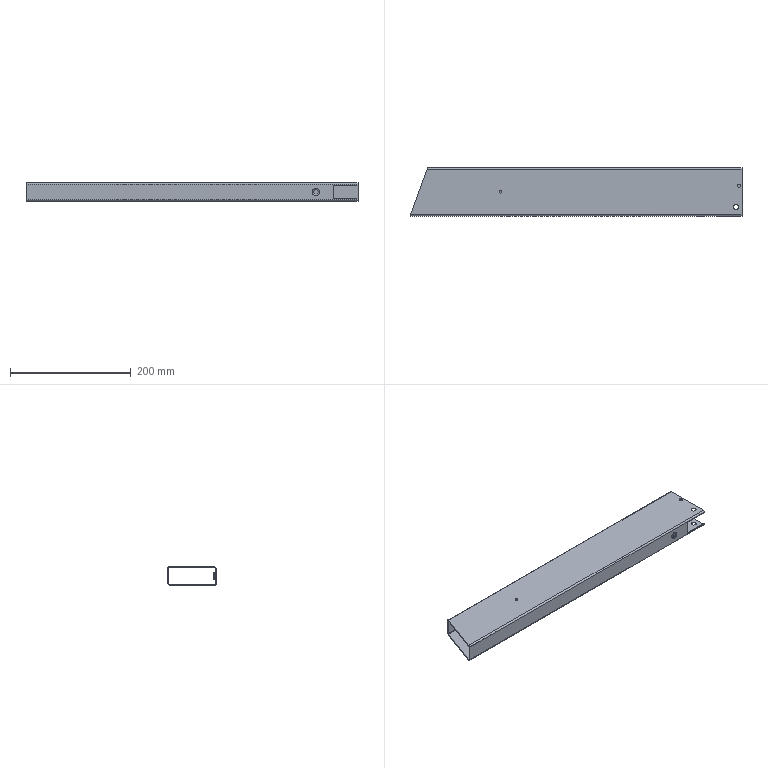Part | STEP file | 7100101 | 1 solid | 29 faces | box 550 x 80 x 30 mm | volume 167922 mm3 | cylinder 14 | plane 14 | torus 1 | commonest cylinder face diameters 5 x5 2 x4 8.5 x2 4 x1 8 x1 11 x1